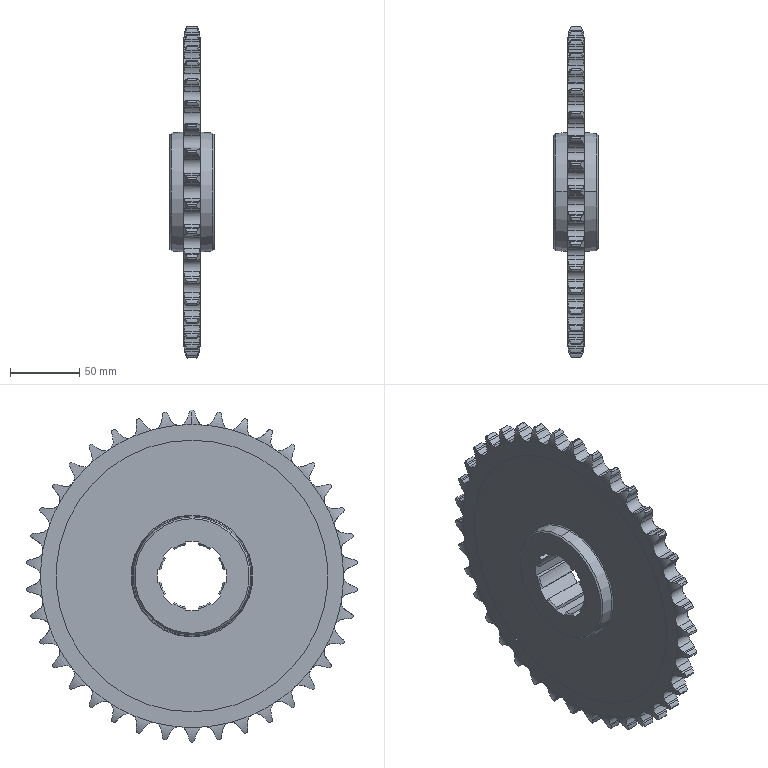Part | SolidWorks | features CirPattern 2, Cut 2, Revolution 2, Chamfer 1, Fillet 1, MirrorPattern 1 | 1 solid | 471 faces | box 32 x 239.32 x 240 mm | volume 513515 mm3 | cylinder 259 | plane 106 | torus 82 | cone 24 | commonest cylinder face diameters 17.009 x80 31.126 x78 12.07 x50 240 x39 46 x8 196.397 x4